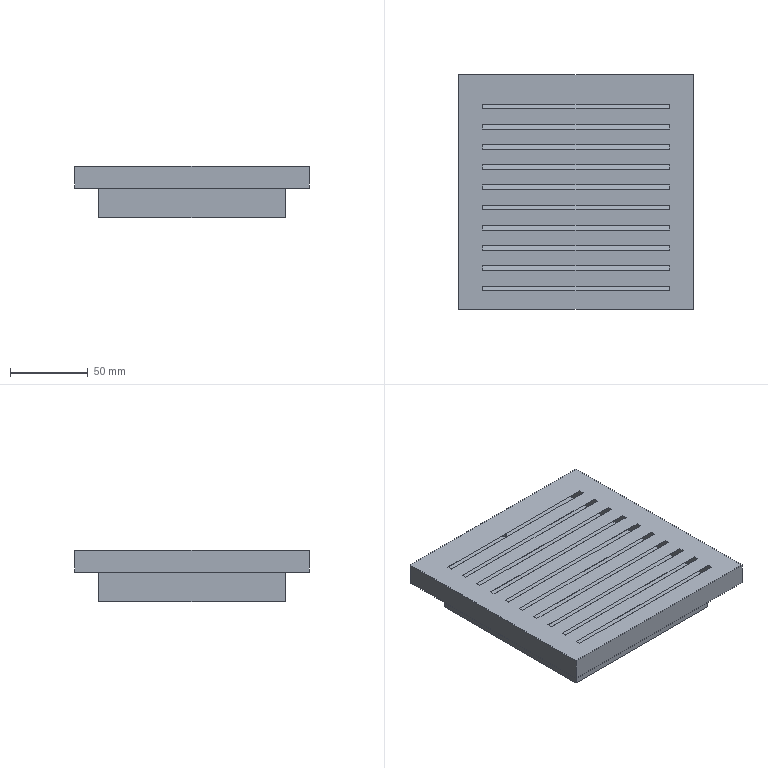Part | STEP file | louvered fan grille LA751PBX0307 | 1 solid | 110 faces | box 151 x 151 x 33 mm | volume 559203 mm3 | plane 61 | cylinder 25 | cone 24 | commonest cylinder face diameters 3.3 x25